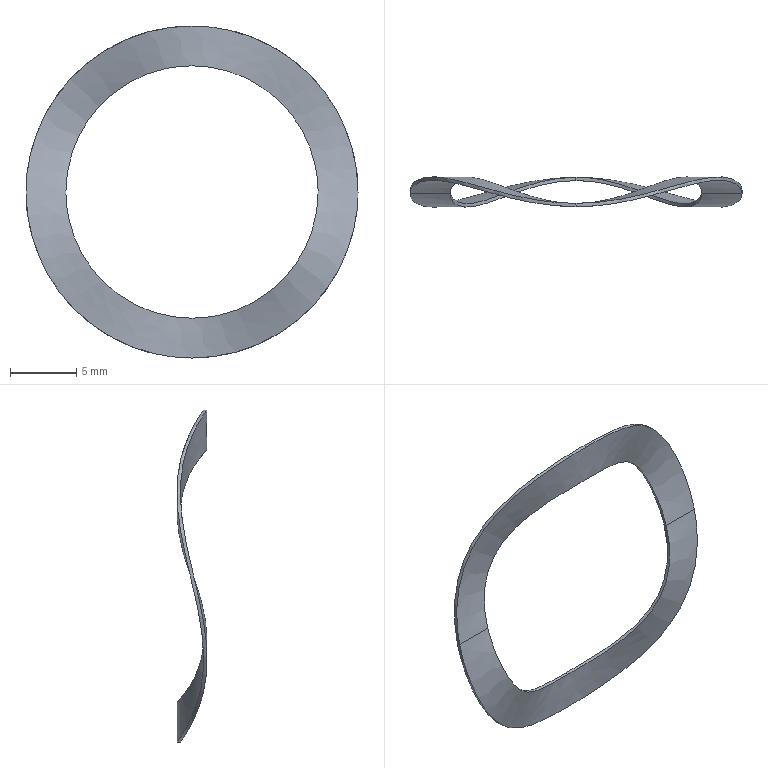Part | STEP file | 1 solid | 8 faces | box 25 x 2.25 x 25 mm | volume 51.836 mm3 | cylinder 4 | spline 4 | commonest cylinder face diameters 19 x2 25 x2